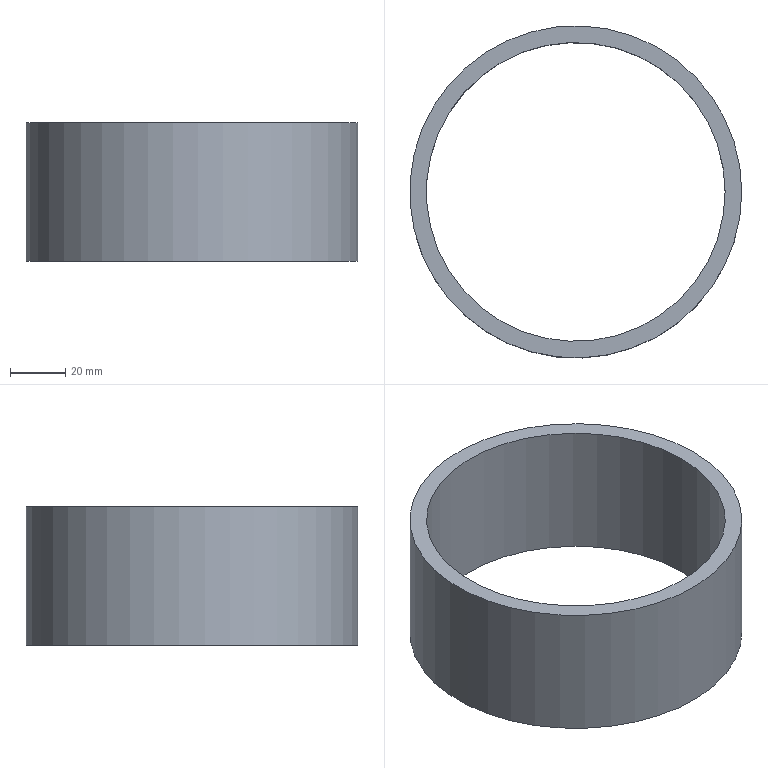Part | NX | features solid 2 | 1 solid | 4 faces | box 120 x 120 x 50 mm | volume 107442 mm3 | cylinder 2 | plane 2 | commonest cylinder face diameters 108 x1 120 x1
STEP:
#1=CARTESIAN_POINT('',(-1231.,595.,-30.));
#2=VERTEX_POINT('',#1);
#3=CARTESIAN_POINT('',(-1285.,595.,-30.));
#4=DIRECTION('',(0.,0.,1.));
#5=DIRECTION('',(1.,0.,0.));
#6=AXIS2_PLACEMENT_3D('',#3,#4,#5);
#7=CIRCLE('',#6,54.);
#8=EDGE_CURVE('',#2,#2,#7,.T.);
#9=ORIENTED_EDGE('',*,*,#8,.F.);
#10=EDGE_LOOP('',(#9));
#11=FACE_BOUND('',#10,.T.);
#12=CARTESIAN_POINT('',(-1231.,595.,20.));
#13=VERTEX_POINT('',#12);
#14=CARTESIAN_POINT('',(-1285.,595.,20.));
#15=DIRECTION('',(0.,0.,1.));
#16=DIRECTION('',(1.,0.,0.));
#17=AXIS2_PLACEMENT_3D('',#14,#15,#16);
#18=CIRCLE('',#17,54.);
#19=EDGE_CURVE('',#13,#13,#18,.T.);
#20=ORIENTED_EDGE('',*,*,#19,.T.);
#21=EDGE_LOOP('',(#20));
#22=FACE_BOUND('',#21,.T.);
#23=CARTESIAN_POINT('',(-1285.,595.,-30.));
#24=DIRECTION('',(0.,0.,1.));
#25=DIRECTION('',(1.,0.,0.));
#26=AXIS2_PLACEMENT_3D('',#23,#24,#25);
#27=CYLINDRICAL_SURFACE('',#26,54.);
#28=ADVANCED_FACE('',(#11,#22),#27,.F.);
#29=CARTESIAN_POINT('',(-1225.,595.,-30.));
#30=VERTEX_POINT('',#29);
#31=CARTESIAN_POINT('',(-1285.,595.,-30.));
#32=DIRECTION('',(0.,0.,1.));
#33=DIRECTION('',(1.,0.,0.));
#34=AXIS2_PLACEMENT_3D('',#31,#32,#33);
#35=CIRCLE('',#34,60.);
#36=EDGE_CURVE('',#30,#30,#35,.T.);
#37=ORIENTED_EDGE('',*,*,#36,.T.);
#38=EDGE_LOOP('',(#37));
#39=FACE_BOUND('',#38,.T.);
#40=CARTESIAN_POINT('',(-1225.,595.,20.));
#41=VERTEX_POINT('',#40);
#42=CARTESIAN_POINT('',(-1285.,595.,20.));
#43=DIRECTION('',(0.,0.,1.));
#44=DIRECTION('',(1.,0.,0.));
#45=AXIS2_PLACEMENT_3D('',#42,#43,#44);
#46=CIRCLE('',#45,60.);
#47=EDGE_CURVE('',#41,#41,#46,.T.);
#48=ORIENTED_EDGE('',*,*,#47,.F.);
#49=EDGE_LOOP('',(#48));
#50=FACE_BOUND('',#49,.T.);
#51=CARTESIAN_POINT('',(-1285.,595.,-30.));
#52=DIRECTION('',(0.,0.,1.));
#53=DIRECTION('',(1.,0.,0.));
#54=AXIS2_PLACEMENT_3D('',#51,#52,#53);
#55=CYLINDRICAL_SURFACE('',#54,60.);
#56=ADVANCED_FACE('',(#39,#50),#55,.T.);
#57=ORIENTED_EDGE('',*,*,#8,.T.);
#58=EDGE_LOOP('',(#57));
#59=FACE_BOUND('',#58,.T.);
#60=ORIENTED_EDGE('',*,*,#36,.F.);
#61=EDGE_LOOP('',(#60));
#62=FACE_BOUND('',#61,.T.);
#63=CARTESIAN_POINT('',(-1285.,595.,-30.));
#64=DIRECTION('',(0.,0.,1.));
#65=DIRECTION('',(-1.,0.,0.));
#66=AXIS2_PLACEMENT_3D('',#63,#64,#65);
#67=PLANE('',#66);
#68=ADVANCED_FACE('',(#59,#62),#67,.F.);
#69=ORIENTED_EDGE('',*,*,#19,.F.);
#70=EDGE_LOOP('',(#69));
#71=FACE_BOUND('',#70,.T.);
#72=ORIENTED_EDGE('',*,*,#47,.T.);
#73=EDGE_LOOP('',(#72));
#74=FACE_BOUND('',#73,.T.);
#75=CARTESIAN_POINT('',(-1285.,595.,20.));
#76=DIRECTION('',(0.,0.,1.));
#77=DIRECTION('',(-1.,0.,0.));
#78=AXIS2_PLACEMENT_3D('',#75,#76,#77);
#79=PLANE('',#78);
#80=ADVANCED_FACE('',(#71,#74),#79,.T.);
#81=CLOSED_SHELL('',(#28,#56,#68,#80));
#82=MANIFOLD_SOLID_BREP('',#81);
#83=(LENGTH_UNIT()NAMED_UNIT(*)SI_UNIT(.MILLI.,.METRE.));
#84=UNCERTAINTY_MEASURE_WITH_UNIT(LENGTH_MEASURE(0.00001),#83,'','');
#85=(NAMED_UNIT(*)PLANE_ANGLE_UNIT()SI_UNIT($,.RADIAN.));
#86=(NAMED_UNIT(*)SI_UNIT($,.STERADIAN.)SOLID_ANGLE_UNIT());
#87=(GEOMETRIC_REPRESENTATION_CONTEXT(3)GLOBAL_UNCERTAINTY_ASSIGNED_CONTEXT((#84))GLOBAL_UNIT_ASSIGNED_CONTEXT((#83,#85,#86))REPRESENTATION_CONTEXT('',''));
#88=ADVANCED_BREP_SHAPE_REPRESENTATION('',(#82),#87);